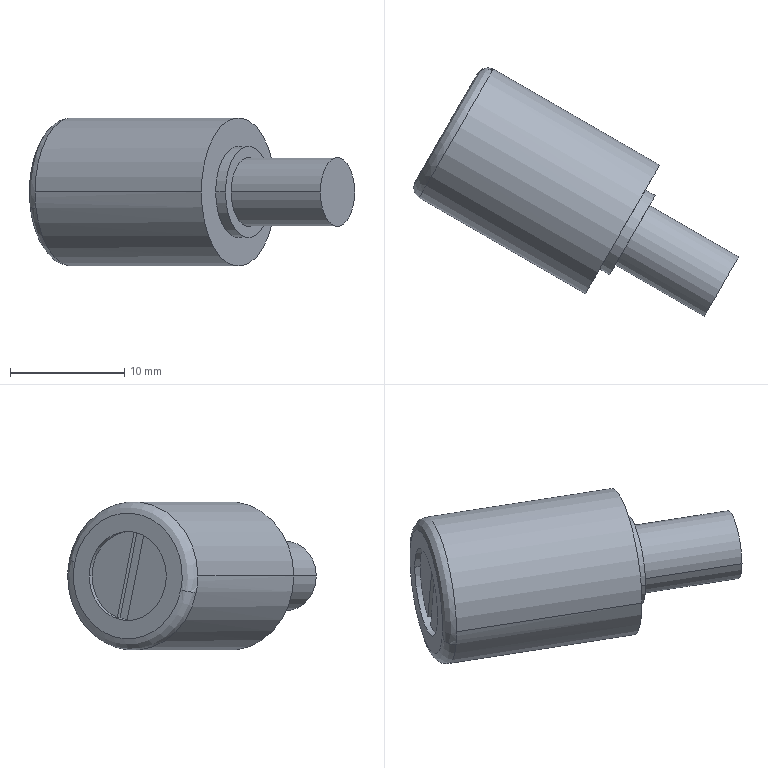Part | SolidWorks | features BaseBody 1 | 1 solid | 19 faces | box 28.459 x 21.761 x 13 mm | volume 2631 mm3 | plane 9 | cylinder 8 | spline 2 | commonest cylinder face diameters 6 x2 7.8 x2 8 x2 13 x2
STEP:
#1=CARTESIAN_POINT('',(-320.378,1833.273,-1193.579));
#2=VERTEX_POINT('',#1);
#3=CARTESIAN_POINT('',(-313.959,1844.392,-1192.141));
#4=VERTEX_POINT('',#3);
#5=CARTESIAN_POINT('',(-317.209,1838.763,-1192.141));
#6=DIRECTION('',(0.866,-0.5,0.));
#7=DIRECTION('',(0.5,0.866,0.));
#8=AXIS2_PLACEMENT_3D('',#5,#6,#7);
#9=CIRCLE('',#8,6.5);
#10=EDGE_CURVE('',#2,#4,#9,.T.);
#11=ORIENTED_EDGE('',*,*,#10,.F.);
#12=CARTESIAN_POINT('',(-320.757,1834.617,-1193.358));
#13=VERTEX_POINT('',#12);
#14=CARTESIAN_POINT('',(-319.891,1834.117,-1193.358));
#15=DIRECTION('',(0.1106,0.1916,-0.9752));
#16=DIRECTION('',(-0.4876,-0.8446,-0.2213));
#17=AXIS2_PLACEMENT_3D('',#14,#15,#16);
#18=CIRCLE('',#17,1.);
#19=EDGE_CURVE('',#2,#13,#18,.T.);
#20=ORIENTED_EDGE('',*,*,#19,.T.);
#21=CARTESIAN_POINT('',(-315.393,1843.908,-1190.924));
#22=VERTEX_POINT('',#21);
#23=CARTESIAN_POINT('',(-320.757,1834.617,-1193.358));
#24=CARTESIAN_POINT('',(-320.4,1835.235,-1196.5));
#25=CARTESIAN_POINT('',(-319.037,1837.595,-1198.217));
#26=CARTESIAN_POINT('',(-317.466,1840.316,-1197.504));
#27=CARTESIAN_POINT('',(-315.895,1843.037,-1196.791));
#28=CARTESIAN_POINT('',(-315.037,1844.525,-1194.066));
#29=CARTESIAN_POINT('',(-315.393,1843.908,-1190.924));
#30=(BOUNDED_CURVE()B_SPLINE_CURVE(3,(#23,#24,#25,#26,#27,#28,#29),.UNSPECIFIED.,.F.,.F.)B_SPLINE_CURVE_WITH_KNOTS((4,3,4),(0.,0.5,1.),.UNSPECIFIED.)CURVE()GEOMETRIC_REPRESENTATION_ITEM()RATIONAL_B_SPLINE_CURVE((1.,0.8047,0.8047,1.,0.8047,0.8047,1.))REPRESENTATION_ITEM(''));
#31=EDGE_CURVE('',#13,#22,#30,.T.);
#32=ORIENTED_EDGE('',*,*,#31,.T.);
#33=CARTESIAN_POINT('',(-314.039,1844.252,-1190.702));
#34=VERTEX_POINT('',#33);
#35=CARTESIAN_POINT('',(-314.527,1843.408,-1190.924));
#36=DIRECTION('',(-0.1106,-0.1916,0.9752));
#37=DIRECTION('',(0.4876,0.8446,0.2213));
#38=AXIS2_PLACEMENT_3D('',#35,#36,#37);
#39=CIRCLE('',#38,1.);
#40=EDGE_CURVE('',#34,#22,#39,.T.);
#41=ORIENTED_EDGE('',*,*,#40,.F.);
#42=CARTESIAN_POINT('',(-317.209,1838.763,-1192.141));
#43=DIRECTION('',(0.866,-0.5,0.));
#44=DIRECTION('',(0.5,0.866,0.));
#45=AXIS2_PLACEMENT_3D('',#42,#43,#44);
#46=CIRCLE('',#45,6.5);
#47=EDGE_CURVE('',#4,#34,#46,.T.);
#48=ORIENTED_EDGE('',*,*,#47,.F.);
#49=EDGE_LOOP('',(#11,#20,#32,#41,#48));
#50=FACE_OUTER_BOUND('',#49,.T.);
#51=CARTESIAN_POINT('',(-320.378,1833.273,-1193.579));
#52=CARTESIAN_POINT('',(-319.957,1834.003,-1197.292));
#53=CARTESIAN_POINT('',(-318.346,1836.792,-1199.322));
#54=CARTESIAN_POINT('',(-316.49,1840.008,-1198.479));
#55=CARTESIAN_POINT('',(-314.633,1843.224,-1197.637));
#56=CARTESIAN_POINT('',(-313.618,1844.982,-1194.416));
#57=CARTESIAN_POINT('',(-314.039,1844.252,-1190.702));
#58=CARTESIAN_POINT('',(-320.886,1833.566,-1193.579));
#59=CARTESIAN_POINT('',(-320.464,1834.295,-1197.292));
#60=CARTESIAN_POINT('',(-318.854,1837.085,-1199.322));
#61=CARTESIAN_POINT('',(-316.997,1840.301,-1198.479));
#62=CARTESIAN_POINT('',(-315.14,1843.517,-1197.637));
#63=CARTESIAN_POINT('',(-314.125,1845.275,-1194.416));
#64=CARTESIAN_POINT('',(-314.547,1844.545,-1190.702));
#65=CARTESIAN_POINT('',(-321.042,1834.123,-1193.487));
#66=CARTESIAN_POINT('',(-320.648,1834.806,-1196.964));
#67=CARTESIAN_POINT('',(-319.14,1837.418,-1198.864));
#68=CARTESIAN_POINT('',(-317.402,1840.429,-1198.076));
#69=CARTESIAN_POINT('',(-315.663,1843.44,-1197.287));
#70=CARTESIAN_POINT('',(-314.713,1845.085,-1194.271));
#71=CARTESIAN_POINT('',(-315.107,1844.402,-1190.794));
#72=CARTESIAN_POINT('',(-320.757,1834.617,-1193.358));
#73=CARTESIAN_POINT('',(-320.4,1835.235,-1196.5));
#74=CARTESIAN_POINT('',(-319.037,1837.595,-1198.217));
#75=CARTESIAN_POINT('',(-317.466,1840.316,-1197.504));
#76=CARTESIAN_POINT('',(-315.895,1843.037,-1196.791));
#77=CARTESIAN_POINT('',(-315.037,1844.525,-1194.066));
#78=CARTESIAN_POINT('',(-315.393,1843.908,-1190.924));
#79=(BOUNDED_SURFACE()B_SPLINE_SURFACE(3,3,((#51,#52,#53,#54,#55,#56,#57),(#58,#59,#60,#61,#62,#63,#64),(#65,#66,#67,#68,#69,#70,#71),(#72,#73,#74,#75,#76,#77,#78)),.UNSPECIFIED.,.F.,.F.,.F.)B_SPLINE_SURFACE_WITH_KNOTS((4,4),(4,3,4),(0.,1.),(0.,0.5,1.),.UNSPECIFIED.)GEOMETRIC_REPRESENTATION_ITEM()RATIONAL_B_SPLINE_SURFACE(((1.,0.8047,0.8047,1.,0.8047,0.8047,1.),(0.8047,0.6476,0.6476,0.8047,0.6476,0.6476,0.8047),(0.8047,0.6476,0.6476,0.8047,0.6476,0.6476,0.8047),(1.,0.8047,0.8047,1.,0.8047,0.8047,1.)))REPRESENTATION_ITEM('')SURFACE());
#80=ADVANCED_FACE('',(#50),#79,.T.);
#81=ORIENTED_EDGE('',*,*,#47,.T.);
#82=CARTESIAN_POINT('',(-320.459,1833.133,-1192.141));
#83=VERTEX_POINT('',#82);
#84=CARTESIAN_POINT('',(-317.209,1838.763,-1192.141));
#85=DIRECTION('',(0.866,-0.5,0.));
#86=DIRECTION('',(0.5,0.866,0.));
#87=AXIS2_PLACEMENT_3D('',#84,#85,#86);
#88=CIRCLE('',#87,6.5);
#89=EDGE_CURVE('',#34,#83,#88,.T.);
#90=ORIENTED_EDGE('',*,*,#89,.T.);
#91=CARTESIAN_POINT('',(-305.91,1824.733,-1192.141));
#92=VERTEX_POINT('',#91);
#93=CARTESIAN_POINT('',(-297.249,1819.733,-1192.141));
#94=DIRECTION('',(0.866,-0.5,0.));
#95=VECTOR('',#94,1000.);
#96=LINE('',#93,#95);
#97=EDGE_CURVE('',#83,#92,#96,.T.);
#98=ORIENTED_EDGE('',*,*,#97,.T.);
#99=CARTESIAN_POINT('',(-299.41,1835.992,-1192.141));
#100=VERTEX_POINT('',#99);
#101=CARTESIAN_POINT('',(-302.66,1830.363,-1192.141));
#102=DIRECTION('',(-0.866,0.5,0.));
#103=DIRECTION('',(0.5,0.866,0.));
#104=AXIS2_PLACEMENT_3D('',#101,#102,#103);
#105=CIRCLE('',#104,6.5);
#106=EDGE_CURVE('',#92,#100,#105,.T.);
#107=ORIENTED_EDGE('',*,*,#106,.T.);
#108=CARTESIAN_POINT('',(-290.749,1830.992,-1192.141));
#109=DIRECTION('',(0.866,-0.5,0.));
#110=VECTOR('',#109,1000.);
#111=LINE('',#108,#110);
#112=EDGE_CURVE('',#4,#100,#111,.T.);
#113=ORIENTED_EDGE('',*,*,#112,.F.);
#114=EDGE_LOOP('',(#81,#90,#98,#107,#113));
#115=FACE_OUTER_BOUND('',#114,.T.);
#116=CARTESIAN_POINT('',(-293.999,1825.363,-1192.141));
#117=DIRECTION('',(0.866,-0.5,0.));
#118=DIRECTION('',(0.5,0.866,0.));
#119=AXIS2_PLACEMENT_3D('',#116,#117,#118);
#120=CYLINDRICAL_SURFACE('',#119,6.5);
#121=ADVANCED_FACE('',(#115),#120,.T.);
#122=CARTESIAN_POINT('',(-304.66,1826.898,-1192.141));
#123=VERTEX_POINT('',#122);
#124=CARTESIAN_POINT('',(-300.66,1833.827,-1192.141));
#125=VERTEX_POINT('',#124);
#126=CARTESIAN_POINT('',(-302.66,1830.363,-1192.141));
#127=DIRECTION('',(-0.866,0.5,0.));
#128=DIRECTION('',(0.5,0.866,0.));
#129=AXIS2_PLACEMENT_3D('',#126,#127,#128);
#130=CIRCLE('',#129,4.);
#131=EDGE_CURVE('',#123,#125,#130,.T.);
#132=ORIENTED_EDGE('',*,*,#131,.F.);
#133=CARTESIAN_POINT('',(-303.794,1826.398,-1192.141));
#134=VERTEX_POINT('',#133);
#135=CARTESIAN_POINT('',(-295.999,1821.898,-1192.141));
#136=DIRECTION('',(0.866,-0.5,0.));
#137=VECTOR('',#136,1000.);
#138=LINE('',#135,#137);
#139=EDGE_CURVE('',#123,#134,#138,.T.);
#140=ORIENTED_EDGE('',*,*,#139,.T.);
#141=CARTESIAN_POINT('',(-299.794,1833.327,-1192.141));
#142=VERTEX_POINT('',#141);
#143=CARTESIAN_POINT('',(-301.794,1829.863,-1192.141));
#144=DIRECTION('',(-0.866,0.5,0.));
#145=DIRECTION('',(0.5,0.866,0.));
#146=AXIS2_PLACEMENT_3D('',#143,#144,#145);
#147=CIRCLE('',#146,4.);
#148=EDGE_CURVE('',#134,#142,#147,.T.);
#149=ORIENTED_EDGE('',*,*,#148,.T.);
#150=CARTESIAN_POINT('',(-291.999,1828.827,-1192.141));
#151=DIRECTION('',(0.866,-0.5,0.));
#152=VECTOR('',#151,1000.);
#153=LINE('',#150,#152);
#154=EDGE_CURVE('',#125,#142,#153,.T.);
#155=ORIENTED_EDGE('',*,*,#154,.F.);
#156=EDGE_LOOP('',(#132,#140,#149,#155));
#157=FACE_OUTER_BOUND('',#156,.T.);
#158=CARTESIAN_POINT('',(-293.999,1825.363,-1192.141));
#159=DIRECTION('',(0.866,-0.5,0.));
#160=DIRECTION('',(0.5,0.866,0.));
#161=AXIS2_PLACEMENT_3D('',#158,#159,#160);
#162=CYLINDRICAL_SURFACE('',#161,4.);
#163=ADVANCED_FACE('',(#157),#162,.T.);
#164=CARTESIAN_POINT('',(-315.692,1842.39,-1192.141));
#165=VERTEX_POINT('',#164);
#166=CARTESIAN_POINT('',(-316.97,1840.176,-1195.802));
#167=VERTEX_POINT('',#166);
#168=CARTESIAN_POINT('',(-317.642,1839.013,-1192.141));
#169=DIRECTION('',(-0.866,0.5,0.));
#170=DIRECTION('',(-0.5,-0.866,0.));
#171=AXIS2_PLACEMENT_3D('',#168,#169,#170);
#172=CIRCLE('',#171,3.9);
#173=EDGE_CURVE('',#165,#167,#172,.T.);
#174=ORIENTED_EDGE('',*,*,#173,.F.);
#175=CARTESIAN_POINT('',(-316.125,1842.64,-1192.141));
#176=VERTEX_POINT('',#175);
#177=CARTESIAN_POINT('',(-315.692,1842.39,-1192.141));
#178=DIRECTION('',(-0.866,0.5,0.));
#179=VECTOR('',#178,1000.);
#180=LINE('',#177,#179);
#181=EDGE_CURVE('',#165,#176,#180,.T.);
#182=ORIENTED_EDGE('',*,*,#181,.T.);
#183=CARTESIAN_POINT('',(-320.025,1835.885,-1192.141));
#184=VERTEX_POINT('',#183);
#185=CARTESIAN_POINT('',(-318.075,1839.263,-1192.141));
#186=DIRECTION('',(0.866,-0.5,0.));
#187=DIRECTION('',(-0.5,-0.866,0.));
#188=AXIS2_PLACEMENT_3D('',#185,#186,#187);
#189=CIRCLE('',#188,3.9);
#190=EDGE_CURVE('',#184,#176,#189,.T.);
#191=ORIENTED_EDGE('',*,*,#190,.F.);
#192=CARTESIAN_POINT('',(-319.592,1835.635,-1192.141));
#193=VERTEX_POINT('',#192);
#194=CARTESIAN_POINT('',(-319.592,1835.635,-1192.141));
#195=DIRECTION('',(-0.866,0.5,0.));
#196=VECTOR('',#195,1000.);
#197=LINE('',#194,#196);
#198=EDGE_CURVE('',#193,#184,#197,.T.);
#199=ORIENTED_EDGE('',*,*,#198,.F.);
#200=CARTESIAN_POINT('',(-317.458,1839.331,-1196.023));
#201=VERTEX_POINT('',#200);
#202=CARTESIAN_POINT('',(-317.642,1839.013,-1192.141));
#203=DIRECTION('',(-0.866,0.5,0.));
#204=DIRECTION('',(-0.5,-0.866,0.));
#205=AXIS2_PLACEMENT_3D('',#202,#203,#204);
#206=CIRCLE('',#205,3.9);
#207=EDGE_CURVE('',#201,#193,#206,.T.);
#208=ORIENTED_EDGE('',*,*,#207,.F.);
#209=CARTESIAN_POINT('',(-317.025,1839.081,-1196.023));
#210=VERTEX_POINT('',#209);
#211=CARTESIAN_POINT('',(-317.458,1839.331,-1196.023));
#212=DIRECTION('',(-0.866,0.5,0.));
#213=VECTOR('',#212,1000.);
#214=LINE('',#211,#213);
#215=EDGE_CURVE('',#210,#201,#214,.T.);
#216=ORIENTED_EDGE('',*,*,#215,.F.);
#217=CARTESIAN_POINT('',(-316.537,1839.926,-1195.802));
#218=VERTEX_POINT('',#217);
#219=CARTESIAN_POINT('',(-317.209,1838.763,-1192.141));
#220=DIRECTION('',(-0.866,0.5,0.));
#221=DIRECTION('',(-0.5,-0.866,0.));
#222=AXIS2_PLACEMENT_3D('',#219,#220,#221);
#223=CIRCLE('',#222,3.9);
#224=EDGE_CURVE('',#218,#210,#223,.T.);
#225=ORIENTED_EDGE('',*,*,#224,.F.);
#226=CARTESIAN_POINT('',(-316.97,1840.176,-1195.802));
#227=DIRECTION('',(0.866,-0.5,0.));
#228=VECTOR('',#227,1000.);
#229=LINE('',#226,#228);
#230=EDGE_CURVE('',#167,#218,#229,.T.);
#231=ORIENTED_EDGE('',*,*,#230,.F.);
#232=EDGE_LOOP('',(#174,#182,#191,#199,#208,#216,#225,#231));
#233=FACE_OUTER_BOUND('',#232,.T.);
#234=CARTESIAN_POINT('',(-317.642,1839.013,-1192.141));
#235=DIRECTION('',(-0.866,0.5,0.));
#236=DIRECTION('',(-0.5,-0.866,0.));
#237=AXIS2_PLACEMENT_3D('',#234,#235,#236);
#238=CYLINDRICAL_SURFACE('',#237,3.9);
#239=ADVANCED_FACE('',(#233),#238,.F.);
#240=CARTESIAN_POINT('',(-303.294,1827.264,-1192.141));
#241=VERTEX_POINT('',#240);
#242=CARTESIAN_POINT('',(-300.294,1832.461,-1192.141));
#243=VERTEX_POINT('',#242);
#244=CARTESIAN_POINT('',(-301.794,1829.863,-1192.141));
#245=DIRECTION('',(-0.866,0.5,0.));
#246=DIRECTION('',(0.5,0.866,0.));
#247=AXIS2_PLACEMENT_3D('',#244,#245,#246);
#248=CIRCLE('',#247,3.);
#249=EDGE_CURVE('',#241,#243,#248,.T.);
#250=ORIENTED_EDGE('',*,*,#249,.F.);
#251=CARTESIAN_POINT('',(-295.499,1822.764,-1192.141));
#252=VERTEX_POINT('',#251);
#253=CARTESIAN_POINT('',(-295.499,1822.764,-1192.141));
#254=DIRECTION('',(0.866,-0.5,0.));
#255=VECTOR('',#254,1000.);
#256=LINE('',#253,#255);
#257=EDGE_CURVE('',#241,#252,#256,.T.);
#258=ORIENTED_EDGE('',*,*,#257,.T.);
#259=CARTESIAN_POINT('',(-292.499,1827.961,-1192.141));
#260=VERTEX_POINT('',#259);
#261=CARTESIAN_POINT('',(-293.999,1825.363,-1192.141));
#262=DIRECTION('',(-0.866,0.5,0.));
#263=DIRECTION('',(0.5,0.866,0.));
#264=AXIS2_PLACEMENT_3D('',#261,#262,#263);
#265=CIRCLE('',#264,3.);
#266=EDGE_CURVE('',#252,#260,#265,.T.);
#267=ORIENTED_EDGE('',*,*,#266,.T.);
#268=CARTESIAN_POINT('',(-292.499,1827.961,-1192.141));
#269=DIRECTION('',(0.866,-0.5,0.));
#270=VECTOR('',#269,1000.);
#271=LINE('',#268,#270);
#272=EDGE_CURVE('',#243,#260,#271,.T.);
#273=ORIENTED_EDGE('',*,*,#272,.F.);
#274=EDGE_LOOP('',(#250,#258,#267,#273));
#275=FACE_OUTER_BOUND('',#274,.T.);
#276=CARTESIAN_POINT('',(-293.999,1825.363,-1192.141));
#277=DIRECTION('',(0.866,-0.5,0.));
#278=DIRECTION('',(0.5,0.866,0.));
#279=AXIS2_PLACEMENT_3D('',#276,#277,#278);
#280=CYLINDRICAL_SURFACE('',#279,3.);
#281=ADVANCED_FACE('',(#275),#280,.T.);
#282=ORIENTED_EDGE('',*,*,#97,.F.);
#283=CARTESIAN_POINT('',(-317.209,1838.763,-1192.141));
#284=DIRECTION('',(0.866,-0.5,0.));
#285=DIRECTION('',(0.5,0.866,0.));
#286=AXIS2_PLACEMENT_3D('',#283,#284,#285);
#287=CIRCLE('',#286,6.5);
#288=EDGE_CURVE('',#83,#2,#287,.T.);
#289=ORIENTED_EDGE('',*,*,#288,.T.);
#290=ORIENTED_EDGE('',*,*,#10,.T.);
#291=ORIENTED_EDGE('',*,*,#112,.T.);
#292=CARTESIAN_POINT('',(-302.66,1830.363,-1192.141));
#293=DIRECTION('',(-0.866,0.5,0.));
#294=DIRECTION('',(0.5,0.866,0.));
#295=AXIS2_PLACEMENT_3D('',#292,#293,#294);
#296=CIRCLE('',#295,6.5);
#297=EDGE_CURVE('',#100,#92,#296,.T.);
#298=ORIENTED_EDGE('',*,*,#297,.T.);
#299=EDGE_LOOP('',(#282,#289,#290,#291,#298));
#300=FACE_OUTER_BOUND('',#299,.T.);
#301=CARTESIAN_POINT('',(-293.999,1825.363,-1192.141));
#302=DIRECTION('',(0.866,-0.5,0.));
#303=DIRECTION('',(0.5,0.866,0.));
#304=AXIS2_PLACEMENT_3D('',#301,#302,#303);
#305=CYLINDRICAL_SURFACE('',#304,6.5);
#306=ADVANCED_FACE('',(#300),#305,.T.);
#307=ORIENTED_EDGE('',*,*,#19,.F.);
#308=ORIENTED_EDGE('',*,*,#288,.F.);
#309=ORIENTED_EDGE('',*,*,#89,.F.);
#310=ORIENTED_EDGE('',*,*,#40,.T.);
#311=CARTESIAN_POINT('',(-315.393,1843.908,-1190.924));
#312=CARTESIAN_POINT('',(-315.749,1843.29,-1187.782));
#313=CARTESIAN_POINT('',(-317.112,1840.93,-1186.064));
#314=CARTESIAN_POINT('',(-318.683,1838.209,-1186.777));
#315=CARTESIAN_POINT('',(-320.254,1835.488,-1187.49));
#316=CARTESIAN_POINT('',(-321.113,1834.,-1190.216));
#317=CARTESIAN_POINT('',(-320.757,1834.617,-1193.358));
#318=(BOUNDED_CURVE()B_SPLINE_CURVE(3,(#311,#312,#313,#314,#315,#316,#317),.UNSPECIFIED.,.F.,.T.)B_SPLINE_CURVE_WITH_KNOTS((4,3,4),(0.,0.5,1.),.UNSPECIFIED.)CURVE()GEOMETRIC_REPRESENTATION_ITEM()RATIONAL_B_SPLINE_CURVE((1.,0.8047,0.8047,1.,0.8047,0.8047,1.))REPRESENTATION_ITEM(''));
#319=EDGE_CURVE('',#22,#13,#318,.T.);
#320=ORIENTED_EDGE('',*,*,#319,.T.);
#321=EDGE_LOOP('',(#307,#308,#309,#310,#320));
#322=FACE_OUTER_BOUND('',#321,.T.);
#323=CARTESIAN_POINT('',(-314.039,1844.252,-1190.702));
#324=CARTESIAN_POINT('',(-314.461,1843.523,-1186.989));
#325=CARTESIAN_POINT('',(-316.071,1840.733,-1184.959));
#326=CARTESIAN_POINT('',(-317.928,1837.517,-1185.802));
#327=CARTESIAN_POINT('',(-319.785,1834.301,-1186.644));
#328=CARTESIAN_POINT('',(-320.799,1832.543,-1189.866));
#329=CARTESIAN_POINT('',(-320.378,1833.273,-1193.579));
#330=CARTESIAN_POINT('',(-314.547,1844.545,-1190.702));
#331=CARTESIAN_POINT('',(-314.968,1843.815,-1186.989));
#332=CARTESIAN_POINT('',(-316.579,1841.026,-1184.959));
#333=CARTESIAN_POINT('',(-318.435,1837.81,-1185.802));
#334=CARTESIAN_POINT('',(-320.292,1834.594,-1186.644));
#335=CARTESIAN_POINT('',(-321.307,1832.836,-1189.866));
#336=CARTESIAN_POINT('',(-320.886,1833.566,-1193.579));
#337=CARTESIAN_POINT('',(-315.107,1844.402,-1190.794));
#338=CARTESIAN_POINT('',(-315.502,1843.719,-1187.317));
#339=CARTESIAN_POINT('',(-317.01,1841.107,-1185.417));
#340=CARTESIAN_POINT('',(-318.748,1838.096,-1186.206));
#341=CARTESIAN_POINT('',(-320.486,1835.086,-1186.994));
#342=CARTESIAN_POINT('',(-321.437,1833.44,-1190.011));
#343=CARTESIAN_POINT('',(-321.042,1834.123,-1193.487));
#344=CARTESIAN_POINT('',(-315.393,1843.908,-1190.924));
#345=CARTESIAN_POINT('',(-315.749,1843.29,-1187.782));
#346=CARTESIAN_POINT('',(-317.112,1840.93,-1186.064));
#347=CARTESIAN_POINT('',(-318.683,1838.209,-1186.777));
#348=CARTESIAN_POINT('',(-320.254,1835.488,-1187.49));
#349=CARTESIAN_POINT('',(-321.113,1834.,-1190.216));
#350=CARTESIAN_POINT('',(-320.757,1834.617,-1193.358));
#351=(BOUNDED_SURFACE()B_SPLINE_SURFACE(3,3,((#323,#324,#325,#326,#327,#328,#329),(#330,#331,#332,#333,#334,#335,#336),(#337,#338,#339,#340,#341,#342,#343),(#344,#345,#346,#347,#348,#349,#350)),.UNSPECIFIED.,.F.,.F.,.F.)B_SPLINE_SURFACE_WITH_KNOTS((4,4),(4,3,4),(0.,1.),(0.,0.5,1.),.UNSPECIFIED.)GEOMETRIC_REPRESENTATION_ITEM()RATIONAL_B_SPLINE_SURFACE(((1.,0.8047,0.8047,1.,0.8047,0.8047,1.),(0.8047,0.6476,0.6476,0.8047,0.6476,0.6476,0.8047),(0.8047,0.6476,0.6476,0.8047,0.6476,0.6476,0.8047),(1.,0.8047,0.8047,1.,0.8047,0.8047,1.)))REPRESENTATION_ITEM('')SURFACE());
#352=ADVANCED_FACE('',(#322),#351,.T.);
#353=CARTESIAN_POINT('',(-302.66,1830.363,-1192.141));
#354=DIRECTION('',(-0.866,0.5,0.));
#355=DIRECTION('',(0.5,0.866,0.));
#356=AXIS2_PLACEMENT_3D('',#353,#354,#355);
#357=CIRCLE('',#356,4.);
#358=EDGE_CURVE('',#125,#123,#357,.T.);
#359=ORIENTED_EDGE('',*,*,#358,.T.);
#360=ORIENTED_EDGE('',*,*,#131,.T.);
#361=EDGE_LOOP('',(#359,#360));
#362=FACE_BOUND('',#361,.T.);
#363=ORIENTED_EDGE('',*,*,#297,.F.);
#364=ORIENTED_EDGE('',*,*,#106,.F.);
#365=EDGE_LOOP('',(#363,#364));
#366=FACE_OUTER_BOUND('',#365,.T.);
#367=CARTESIAN_POINT('',(-303.102,1829.596,-1188.24));
#368=DIRECTION('',(0.866,-0.5,0.));
#369=DIRECTION('',(0.5,0.866,0.));
#370=AXIS2_PLACEMENT_3D('',#367,#368,#369);
#371=PLANE('',#370);
#372=ADVANCED_FACE('',(#362,#366),#371,.T.);
#373=ORIENTED_EDGE('',*,*,#139,.F.);
#374=ORIENTED_EDGE('',*,*,#358,.F.);
#375=ORIENTED_EDGE('',*,*,#154,.T.);
#376=CARTESIAN_POINT('',(-301.794,1829.863,-1192.141));
#377=DIRECTION('',(-0.866,0.5,0.));
#378=DIRECTION('',(0.5,0.866,0.));
#379=AXIS2_PLACEMENT_3D('',#376,#377,#378);
#380=CIRCLE('',#379,4.);
#381=EDGE_CURVE('',#142,#134,#380,.T.);
#382=ORIENTED_EDGE('',*,*,#381,.T.);
#383=EDGE_LOOP('',(#373,#374,#375,#382));
#384=FACE_OUTER_BOUND('',#383,.T.);
#385=CARTESIAN_POINT('',(-293.999,1825.363,-1192.141));
#386=DIRECTION('',(0.866,-0.5,0.));
#387=DIRECTION('',(0.5,0.866,0.));
#388=AXIS2_PLACEMENT_3D('',#385,#386,#387);
#389=CYLINDRICAL_SURFACE('',#388,4.);
#390=ADVANCED_FACE('',(#384),#389,.T.);
#391=ORIENTED_EDGE('',*,*,#190,.T.);
#392=CARTESIAN_POINT('',(-318.075,1839.263,-1192.141));
#393=DIRECTION('',(0.866,-0.5,0.));
#394=DIRECTION('',(-0.5,-0.866,0.));
#395=AXIS2_PLACEMENT_3D('',#392,#393,#394);
#396=CIRCLE('',#395,3.9);
#397=EDGE_CURVE('',#176,#184,#396,.T.);
#398=ORIENTED_EDGE('',*,*,#397,.T.);
#399=EDGE_LOOP('',(#391,#398));
#400=FACE_BOUND('',#399,.T.);
#401=ORIENTED_EDGE('',*,*,#319,.F.);
#402=ORIENTED_EDGE('',*,*,#31,.F.);
#403=EDGE_LOOP('',(#401,#402));
#404=FACE_OUTER_BOUND('',#403,.T.);
#405=CARTESIAN_POINT('',(-318.683,1838.209,-1186.777));
#406=DIRECTION('',(-0.866,0.5,0.));
#407=DIRECTION('',(-0.5,-0.866,0.));
#408=AXIS2_PLACEMENT_3D('',#405,#406,#407);
#409=PLANE('',#408);
#410=ADVANCED_FACE('',(#400,#404),#409,.T.);
#411=CARTESIAN_POINT('',(-301.794,1829.863,-1192.141));
#412=DIRECTION('',(-0.866,0.5,0.));
#413=DIRECTION('',(0.5,0.866,0.));
#414=AXIS2_PLACEMENT_3D('',#411,#412,#413);
#415=CIRCLE('',#414,3.);
#416=EDGE_CURVE('',#243,#241,#415,.T.);
#417=ORIENTED_EDGE('',*,*,#416,.T.);
#418=ORIENTED_EDGE('',*,*,#249,.T.);
#419=EDGE_LOOP('',(#417,#418));
#420=FACE_BOUND('',#419,.T.);
#421=ORIENTED_EDGE('',*,*,#381,.F.);
#422=ORIENTED_EDGE('',*,*,#148,.F.);
#423=EDGE_LOOP('',(#421,#422));
#424=FACE_OUTER_BOUND('',#423,.T.);
#425=CARTESIAN_POINT('',(-302.125,1829.288,-1189.215));
#426=DIRECTION('',(0.866,-0.5,0.));
#427=DIRECTION('',(0.5,0.866,0.));
#428=AXIS2_PLACEMENT_3D('',#425,#426,#427);
#429=PLANE('',#428);
#430=ADVANCED_FACE('',(#420,#424),#429,.T.);
#431=ORIENTED_EDGE('',*,*,#181,.F.);
#432=CARTESIAN_POINT('',(-317.826,1838.694,-1188.258));
#433=VERTEX_POINT('',#432);
#434=CARTESIAN_POINT('',(-317.642,1839.013,-1192.141));
#435=DIRECTION('',(-0.866,0.5,0.));
#436=DIRECTION('',(-0.5,-0.866,0.));
#437=AXIS2_PLACEMENT_3D('',#434,#435,#436);
#438=CIRCLE('',#437,3.9);
#439=EDGE_CURVE('',#433,#165,#438,.T.);
#440=ORIENTED_EDGE('',*,*,#439,.F.);
#441=CARTESIAN_POINT('',(-317.393,1838.444,-1188.258));
#442=VERTEX_POINT('',#441);
#443=CARTESIAN_POINT('',(-317.826,1838.694,-1188.258));
#444=DIRECTION('',(-0.866,0.5,0.));
#445=VECTOR('',#444,1000.);
#446=LINE('',#443,#445);
#447=EDGE_CURVE('',#442,#433,#446,.T.);
#448=ORIENTED_EDGE('',*,*,#447,.F.);
#449=CARTESIAN_POINT('',(-317.88,1837.599,-1188.479));
#450=VERTEX_POINT('',#449);
#451=CARTESIAN_POINT('',(-317.209,1838.763,-1192.141));
#452=DIRECTION('',(-0.866,0.5,0.));
#453=DIRECTION('',(-0.5,-0.866,0.));
#454=AXIS2_PLACEMENT_3D('',#451,#452,#453);
#455=CIRCLE('',#454,3.9);
#456=EDGE_CURVE('',#450,#442,#455,.T.);
#457=ORIENTED_EDGE('',*,*,#456,.F.);
#458=CARTESIAN_POINT('',(-318.314,1837.849,-1188.479));
#459=VERTEX_POINT('',#458);
#460=CARTESIAN_POINT('',(-318.314,1837.849,-1188.479));
#461=DIRECTION('',(0.866,-0.5,0.));
#462=VECTOR('',#461,1000.);
#463=LINE('',#460,#462);
#464=EDGE_CURVE('',#459,#450,#463,.T.);
#465=ORIENTED_EDGE('',*,*,#464,.F.);
#466=CARTESIAN_POINT('',(-317.642,1839.013,-1192.141));
#467=DIRECTION('',(-0.866,0.5,0.));
#468=DIRECTION('',(-0.5,-0.866,0.));
#469=AXIS2_PLACEMENT_3D('',#466,#467,#468);
#470=CIRCLE('',#469,3.9);
#471=EDGE_CURVE('',#193,#459,#470,.T.);
#472=ORIENTED_EDGE('',*,*,#471,.F.);
#473=ORIENTED_EDGE('',*,*,#198,.T.);
#474=ORIENTED_EDGE('',*,*,#397,.F.);
#475=EDGE_LOOP('',(#431,#440,#448,#457,#465,#472,#473,#474));
#476=FACE_OUTER_BOUND('',#475,.T.);
#477=CARTESIAN_POINT('',(-317.642,1839.013,-1192.141));
#478=DIRECTION('',(-0.866,0.5,0.));
#479=DIRECTION('',(-0.5,-0.866,0.));
#480=AXIS2_PLACEMENT_3D('',#477,#478,#479);
#481=CYLINDRICAL_SURFACE('',#480,3.9);
#482=ADVANCED_FACE('',(#476),#481,.F.);
#483=ORIENTED_EDGE('',*,*,#257,.F.);
#484=ORIENTED_EDGE('',*,*,#416,.F.);
#485=ORIENTED_EDGE('',*,*,#272,.T.);
#486=CARTESIAN_POINT('',(-293.999,1825.363,-1192.141));
#487=DIRECTION('',(-0.866,0.5,0.));
#488=DIRECTION('',(0.5,0.866,0.));
#489=AXIS2_PLACEMENT_3D('',#486,#487,#488);
#490=CIRCLE('',#489,3.);
#491=EDGE_CURVE('',#260,#252,#490,.T.);
#492=ORIENTED_EDGE('',*,*,#491,.T.);
#493=EDGE_LOOP('',(#483,#484,#485,#492));
#494=FACE_OUTER_BOUND('',#493,.T.);
#495=CARTESIAN_POINT('',(-293.999,1825.363,-1192.141));
#496=DIRECTION('',(0.866,-0.5,0.));
#497=DIRECTION('',(0.5,0.866,0.));
#498=AXIS2_PLACEMENT_3D('',#495,#496,#497);
#499=CYLINDRICAL_SURFACE('',#498,3.);
#500=ADVANCED_FACE('',(#494),#499,.T.);
#501=ORIENTED_EDGE('',*,*,#439,.T.);
#502=ORIENTED_EDGE('',*,*,#173,.T.);
#503=CARTESIAN_POINT('',(-317.826,1838.694,-1188.258));
#504=DIRECTION('',(0.1106,0.1916,-0.9752));
#505=VECTOR('',#504,1000.);
#506=LINE('',#503,#505);
#507=EDGE_CURVE('',#433,#167,#506,.T.);
#508=ORIENTED_EDGE('',*,*,#507,.F.);
#509=EDGE_LOOP('',(#501,#502,#508));
#510=FACE_OUTER_BOUND('',#509,.T.);
#511=CARTESIAN_POINT('',(-317.642,1839.013,-1192.141));
#512=DIRECTION('',(0.866,-0.5,0.));
#513=DIRECTION('',(0.5,0.866,0.));
#514=AXIS2_PLACEMENT_3D('',#511,#512,#513);
#515=PLANE('',#514);
#516=ADVANCED_FACE('',(#510),#515,.F.);
#517=ORIENTED_EDGE('',*,*,#447,.T.);
#518=ORIENTED_EDGE('',*,*,#507,.T.);
#519=ORIENTED_EDGE('',*,*,#230,.T.);
#520=CARTESIAN_POINT('',(-317.393,1838.444,-1188.258));
#521=DIRECTION('',(-0.1106,-0.1916,0.9752));
#522=VECTOR('',#521,1000.);
#523=LINE('',#520,#522);
#524=EDGE_CURVE('',#218,#442,#523,.T.);
#525=ORIENTED_EDGE('',*,*,#524,.T.);
#526=EDGE_LOOP('',(#517,#518,#519,#525));
#527=FACE_OUTER_BOUND('',#526,.T.);
#528=CARTESIAN_POINT('',(-317.393,1838.444,-1188.258));
#529=DIRECTION('',(-0.4876,-0.8446,-0.2213));
#530=DIRECTION('',(0.866,-0.5,0.));
#531=AXIS2_PLACEMENT_3D('',#528,#529,#530);
#532=PLANE('',#531);
#533=ADVANCED_FACE('',(#527),#532,.T.);
#534=ORIENTED_EDGE('',*,*,#224,.T.);
#535=CARTESIAN_POINT('',(-317.88,1837.599,-1188.479));
#536=DIRECTION('',(0.1106,0.1916,-0.9752));
#537=VECTOR('',#536,1000.);
#538=LINE('',#535,#537);
#539=EDGE_CURVE('',#450,#210,#538,.T.);
#540=ORIENTED_EDGE('',*,*,#539,.F.);
#541=ORIENTED_EDGE('',*,*,#456,.T.);
#542=ORIENTED_EDGE('',*,*,#524,.F.);
#543=EDGE_LOOP('',(#534,#540,#541,#542));
#544=FACE_OUTER_BOUND('',#543,.T.);
#545=CARTESIAN_POINT('',(-317.209,1838.763,-1192.141));
#546=DIRECTION('',(0.866,-0.5,0.));
#547=DIRECTION('',(0.5,0.866,0.));
#548=AXIS2_PLACEMENT_3D('',#545,#546,#547);
#549=PLANE('',#548);
#550=ADVANCED_FACE('',(#544),#549,.F.);
#551=ORIENTED_EDGE('',*,*,#215,.T.);
#552=CARTESIAN_POINT('',(-318.314,1837.849,-1188.479));
#553=DIRECTION('',(-0.1106,-0.1916,0.9752));
#554=VECTOR('',#553,1000.);
#555=LINE('',#552,#554);
#556=EDGE_CURVE('',#201,#459,#555,.T.);
#557=ORIENTED_EDGE('',*,*,#556,.T.);
#558=ORIENTED_EDGE('',*,*,#464,.T.);
#559=ORIENTED_EDGE('',*,*,#539,.T.);
#560=EDGE_LOOP('',(#551,#557,#558,#559));
#561=FACE_OUTER_BOUND('',#560,.T.);
#562=CARTESIAN_POINT('',(-317.88,1837.599,-1188.479));
#563=DIRECTION('',(0.4876,0.8446,0.2213));
#564=DIRECTION('',(-0.866,0.5,0.));
#565=AXIS2_PLACEMENT_3D('',#562,#563,#564);
#566=PLANE('',#565);
#567=ADVANCED_FACE('',(#561),#566,.T.);
#568=ORIENTED_EDGE('',*,*,#207,.T.);
#569=ORIENTED_EDGE('',*,*,#471,.T.);
#570=ORIENTED_EDGE('',*,*,#556,.F.);
#571=EDGE_LOOP('',(#568,#569,#570));
#572=FACE_OUTER_BOUND('',#571,.T.);
#573=CARTESIAN_POINT('',(-317.642,1839.013,-1192.141));
#574=DIRECTION('',(0.866,-0.5,0.));
#575=DIRECTION('',(0.5,0.866,0.));
#576=AXIS2_PLACEMENT_3D('',#573,#574,#575);
#577=PLANE('',#576);
#578=ADVANCED_FACE('',(#572),#577,.F.);
#579=ORIENTED_EDGE('',*,*,#491,.F.);
#580=ORIENTED_EDGE('',*,*,#266,.F.);
#581=EDGE_LOOP('',(#579,#580));
#582=FACE_OUTER_BOUND('',#581,.T.);
#583=CARTESIAN_POINT('',(-293.999,1825.363,-1192.141));
#584=DIRECTION('',(0.866,-0.5,0.));
#585=DIRECTION('',(0.5,0.866,0.));
#586=AXIS2_PLACEMENT_3D('',#583,#584,#585);
#587=PLANE('',#586);
#588=ADVANCED_FACE('',(#582),#587,.T.);
#589=CLOSED_SHELL('',(#80,#121,#163,#239,#281,#306,#352,#372,#390,#410,#430,#482,#500,#516,#533,#550,#567,#578,#588));
#590=MANIFOLD_SOLID_BREP('',#589);
#591=CARTESIAN_POINT('',(0.,0.,0.));
#592=DIRECTION('',(0.,0.,1.));
#593=DIRECTION('',(1.,0.,0.));
#594=AXIS2_PLACEMENT_3D('',#591,#592,#593);
#595=(LENGTH_UNIT()NAMED_UNIT(*)SI_UNIT(.MILLI.,.METRE.));
#596=UNCERTAINTY_MEASURE_WITH_UNIT(LENGTH_MEASURE(0.00001),#595,'','');
#597=(NAMED_UNIT(*)PLANE_ANGLE_UNIT()SI_UNIT($,.RADIAN.));
#598=(NAMED_UNIT(*)SI_UNIT($,.STERADIAN.)SOLID_ANGLE_UNIT());
#599=(GEOMETRIC_REPRESENTATION_CONTEXT(3)GLOBAL_UNCERTAINTY_ASSIGNED_CONTEXT((#596))GLOBAL_UNIT_ASSIGNED_CONTEXT((#595,#597,#598))REPRESENTATION_CONTEXT('',''));
#600=ADVANCED_BREP_SHAPE_REPRESENTATION('',(#590,#594),#599);